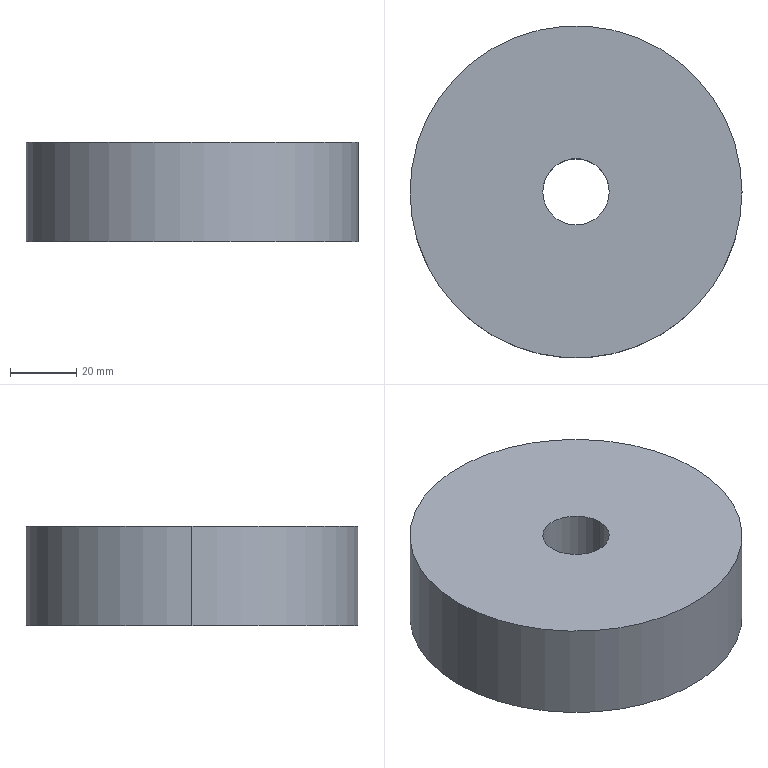Part | STEP file | 1 solid | 6 faces | box 100 x 100 x 30 mm | volume 226195 mm3 | cylinder 4 | plane 2 | commonest cylinder face diameters 20 x2 100 x2
STEP:
#1=CARTESIAN_POINT('',(0.,0.,0.));
#2=DIRECTION('',(0.,0.,1.));
#3=DIRECTION('',(1.,0.,0.));
#4=AXIS2_PLACEMENT_3D('',#1,#2,#3);
#5=CARTESIAN_POINT('',(50.,0.,-15.));
#6=VERTEX_POINT('',#5);
#7=CARTESIAN_POINT('',(-50.,0.,-15.));
#8=VERTEX_POINT('',#7);
#9=CARTESIAN_POINT('',(0.,0.,-15.));
#10=DIRECTION('',(0.,0.,1.));
#11=DIRECTION('',(1.,0.,0.));
#12=AXIS2_PLACEMENT_3D('',#9,#10,#11);
#13=CIRCLE('',#12,50.);
#14=CARTESIAN_POINT('',(0.,0.,0.));
#15=DIRECTION('',(0.,0.,1.));
#16=DIRECTION('',(1.,0.,0.));
#17=AXIS2_PLACEMENT_3D('',#14,#15,#16);
#18=CYLINDRICAL_SURFACE('',#17,50.);
#19=CARTESIAN_POINT('',(0.,-15.));
#20=DIRECTION('',(1.,0.));
#21=VECTOR('',#20,1.);
#22=LINE('',#19,#21);
#23=(GEOMETRIC_REPRESENTATION_CONTEXT(2)PARAMETRIC_REPRESENTATION_CONTEXT()REPRESENTATION_CONTEXT('',''));
#24=DEFINITIONAL_REPRESENTATION('',(#22),#23);
#25=PCURVE('',#18,#24);
#26=CARTESIAN_POINT('',(0.,0.,-15.));
#27=DIRECTION('',(0.,0.,1.));
#28=DIRECTION('',(1.,0.,0.));
#29=AXIS2_PLACEMENT_3D('',#26,#27,#28);
#30=PLANE('',#29);
#31=CARTESIAN_POINT('',(0.,0.));
#32=DIRECTION('',(1.,0.));
#33=AXIS2_PLACEMENT_2D('',#31,#32);
#34=CIRCLE('',#33,50.);
#35=(GEOMETRIC_REPRESENTATION_CONTEXT(2)PARAMETRIC_REPRESENTATION_CONTEXT()REPRESENTATION_CONTEXT('',''));
#36=DEFINITIONAL_REPRESENTATION('',(#34),#35);
#37=PCURVE('',#30,#36);
#38=SURFACE_CURVE('',#13,(#25,#37),.PCURVE_S1.);
#39=EDGE_CURVE('',#6,#8,#38,.T.);
#40=ORIENTED_EDGE('',*,*,#39,.T.);
#41=CARTESIAN_POINT('',(-50.,0.,15.));
#42=VERTEX_POINT('',#41);
#43=CARTESIAN_POINT('',(-50.,0.,0.));
#44=DIRECTION('',(0.,0.,1.));
#45=VECTOR('',#44,1.);
#46=LINE('',#43,#45);
#47=CARTESIAN_POINT('',(3.142,0.));
#48=DIRECTION('',(0.,1.));
#49=VECTOR('',#48,1.);
#50=LINE('',#47,#49);
#51=(GEOMETRIC_REPRESENTATION_CONTEXT(2)PARAMETRIC_REPRESENTATION_CONTEXT()REPRESENTATION_CONTEXT('',''));
#52=DEFINITIONAL_REPRESENTATION('',(#50),#51);
#53=PCURVE('',#18,#52);
#54=CARTESIAN_POINT('',(0.,0.,0.));
#55=DIRECTION('',(0.,0.,1.));
#56=DIRECTION('',(1.,0.,0.));
#57=AXIS2_PLACEMENT_3D('',#54,#55,#56);
#58=CYLINDRICAL_SURFACE('',#57,50.);
#59=CARTESIAN_POINT('',(3.142,0.));
#60=DIRECTION('',(0.,1.));
#61=VECTOR('',#60,1.);
#62=LINE('',#59,#61);
#63=(GEOMETRIC_REPRESENTATION_CONTEXT(2)PARAMETRIC_REPRESENTATION_CONTEXT()REPRESENTATION_CONTEXT('',''));
#64=DEFINITIONAL_REPRESENTATION('',(#62),#63);
#65=PCURVE('',#58,#64);
#66=SURFACE_CURVE('',#46,(#53,#65),.PCURVE_S1.);
#67=EDGE_CURVE('',#8,#42,#66,.T.);
#68=ORIENTED_EDGE('',*,*,#67,.T.);
#69=CARTESIAN_POINT('',(50.,0.,15.));
#70=VERTEX_POINT('',#69);
#71=CARTESIAN_POINT('',(0.,0.,15.));
#72=DIRECTION('',(0.,0.,-1.));
#73=DIRECTION('',(1.,0.,0.));
#74=AXIS2_PLACEMENT_3D('',#71,#72,#73);
#75=CIRCLE('',#74,50.);
#76=CARTESIAN_POINT('',(6.283,15.));
#77=DIRECTION('',(-1.,0.));
#78=VECTOR('',#77,1.);
#79=LINE('',#76,#78);
#80=(GEOMETRIC_REPRESENTATION_CONTEXT(2)PARAMETRIC_REPRESENTATION_CONTEXT()REPRESENTATION_CONTEXT('',''));
#81=DEFINITIONAL_REPRESENTATION('',(#79),#80);
#82=PCURVE('',#18,#81);
#83=CARTESIAN_POINT('',(0.,0.,15.));
#84=DIRECTION('',(0.,0.,1.));
#85=DIRECTION('',(1.,0.,0.));
#86=AXIS2_PLACEMENT_3D('',#83,#84,#85);
#87=PLANE('',#86);
#88=CARTESIAN_POINT('',(50.,0.));
#89=CARTESIAN_POINT('',(50.,-86.603));
#90=CARTESIAN_POINT('',(-25.,-43.301));
#91=CARTESIAN_POINT('',(-100.,0.));
#92=CARTESIAN_POINT('',(-25.,43.301));
#93=CARTESIAN_POINT('',(50.,86.603));
#94=CARTESIAN_POINT('',(50.,0.));
#95=(BOUNDED_CURVE()B_SPLINE_CURVE(2,(#88,#89,#90,#91,#92,#93,#94),.UNSPECIFIED.,.T.,.F.)B_SPLINE_CURVE_WITH_KNOTS((1,2,2,2,2,1),(-2.094,0.,2.094,4.189,6.283,8.378),.UNSPECIFIED.)CURVE()GEOMETRIC_REPRESENTATION_ITEM()RATIONAL_B_SPLINE_CURVE((1.,0.5,1.,0.5,1.,0.5,1.))REPRESENTATION_ITEM(''));
#96=(GEOMETRIC_REPRESENTATION_CONTEXT(2)PARAMETRIC_REPRESENTATION_CONTEXT()REPRESENTATION_CONTEXT('',''));
#97=DEFINITIONAL_REPRESENTATION('',(#95),#96);
#98=PCURVE('',#87,#97);
#99=SURFACE_CURVE('',#75,(#82,#98),.PCURVE_S1.);
#100=EDGE_CURVE('',#42,#70,#99,.T.);
#101=ORIENTED_EDGE('',*,*,#100,.T.);
#102=CARTESIAN_POINT('',(50.,0.,0.));
#103=DIRECTION('',(0.,0.,1.));
#104=VECTOR('',#103,1.);
#105=LINE('',#102,#104);
#106=CARTESIAN_POINT('',(0.,0.));
#107=DIRECTION('',(0.,1.));
#108=VECTOR('',#107,1.);
#109=LINE('',#106,#108);
#110=(GEOMETRIC_REPRESENTATION_CONTEXT(2)PARAMETRIC_REPRESENTATION_CONTEXT()REPRESENTATION_CONTEXT('',''));
#111=DEFINITIONAL_REPRESENTATION('',(#109),#110);
#112=PCURVE('',#18,#111);
#113=CARTESIAN_POINT('',(6.283,0.));
#114=DIRECTION('',(0.,1.));
#115=VECTOR('',#114,1.);
#116=LINE('',#113,#115);
#117=(GEOMETRIC_REPRESENTATION_CONTEXT(2)PARAMETRIC_REPRESENTATION_CONTEXT()REPRESENTATION_CONTEXT('',''));
#118=DEFINITIONAL_REPRESENTATION('',(#116),#117);
#119=PCURVE('',#58,#118);
#120=SURFACE_CURVE('',#105,(#112,#119),.PCURVE_S1.);
#121=EDGE_CURVE('',#6,#70,#120,.T.);
#122=ORIENTED_EDGE('',*,*,#121,.F.);
#123=EDGE_LOOP('',(#40,#68,#101,#122));
#124=FACE_BOUND('',#123,.T.);
#125=ADVANCED_FACE('',(#124),#18,.T.);
#126=CARTESIAN_POINT('',(-10.,0.,15.));
#127=VERTEX_POINT('',#126);
#128=CARTESIAN_POINT('',(-10.,0.,-15.));
#129=VERTEX_POINT('',#128);
#130=CARTESIAN_POINT('',(-10.,0.,15.));
#131=DIRECTION('',(0.,0.,-1.));
#132=VECTOR('',#131,1.);
#133=LINE('',#130,#132);
#134=CARTESIAN_POINT('',(0.,0.,15.));
#135=DIRECTION('',(0.,0.,-1.));
#136=DIRECTION('',(-1.,0.,0.));
#137=AXIS2_PLACEMENT_3D('',#134,#135,#136);
#138=CYLINDRICAL_SURFACE('',#137,10.);
#139=CARTESIAN_POINT('',(6.283,0.));
#140=DIRECTION('',(0.,1.));
#141=VECTOR('',#140,1.);
#142=LINE('',#139,#141);
#143=(GEOMETRIC_REPRESENTATION_CONTEXT(2)PARAMETRIC_REPRESENTATION_CONTEXT()REPRESENTATION_CONTEXT('',''));
#144=DEFINITIONAL_REPRESENTATION('',(#142),#143);
#145=PCURVE('',#138,#144);
#146=CARTESIAN_POINT('',(0.,0.,15.));
#147=DIRECTION('',(0.,0.,-1.));
#148=DIRECTION('',(-1.,0.,0.));
#149=AXIS2_PLACEMENT_3D('',#146,#147,#148);
#150=CYLINDRICAL_SURFACE('',#149,10.);
#151=CARTESIAN_POINT('',(0.,0.));
#152=DIRECTION('',(0.,1.));
#153=VECTOR('',#152,1.);
#154=LINE('',#151,#153);
#155=(GEOMETRIC_REPRESENTATION_CONTEXT(2)PARAMETRIC_REPRESENTATION_CONTEXT()REPRESENTATION_CONTEXT('',''));
#156=DEFINITIONAL_REPRESENTATION('',(#154),#155);
#157=PCURVE('',#150,#156);
#158=SURFACE_CURVE('',#133,(#145,#157),.PCURVE_S1.);
#159=EDGE_CURVE('',#127,#129,#158,.T.);
#160=ORIENTED_EDGE('',*,*,#159,.T.);
#161=CARTESIAN_POINT('',(10.,0.,-15.));
#162=VERTEX_POINT('',#161);
#163=CARTESIAN_POINT('',(0.,0.,-15.));
#164=DIRECTION('',(0.,0.,-1.));
#165=DIRECTION('',(-1.,0.,0.));
#166=AXIS2_PLACEMENT_3D('',#163,#164,#165);
#167=CIRCLE('',#166,10.);
#168=CARTESIAN_POINT('',(0.,30.));
#169=DIRECTION('',(1.,0.));
#170=VECTOR('',#169,1.);
#171=LINE('',#168,#170);
#172=(GEOMETRIC_REPRESENTATION_CONTEXT(2)PARAMETRIC_REPRESENTATION_CONTEXT()REPRESENTATION_CONTEXT('',''));
#173=DEFINITIONAL_REPRESENTATION('',(#171),#172);
#174=PCURVE('',#138,#173);
#175=CARTESIAN_POINT('',(-10.,0.));
#176=CARTESIAN_POINT('',(-10.,17.321));
#177=CARTESIAN_POINT('',(5.,8.66));
#178=CARTESIAN_POINT('',(20.,0.));
#179=CARTESIAN_POINT('',(5.,-8.66));
#180=CARTESIAN_POINT('',(-10.,-17.321));
#181=CARTESIAN_POINT('',(-10.,0.));
#182=(BOUNDED_CURVE()B_SPLINE_CURVE(2,(#175,#176,#177,#178,#179,#180,#181),.UNSPECIFIED.,.T.,.F.)B_SPLINE_CURVE_WITH_KNOTS((1,2,2,2,2,1),(-2.094,0.,2.094,4.189,6.283,8.378),.UNSPECIFIED.)CURVE()GEOMETRIC_REPRESENTATION_ITEM()RATIONAL_B_SPLINE_CURVE((1.,0.5,1.,0.5,1.,0.5,1.))REPRESENTATION_ITEM(''));
#183=(GEOMETRIC_REPRESENTATION_CONTEXT(2)PARAMETRIC_REPRESENTATION_CONTEXT()REPRESENTATION_CONTEXT('',''));
#184=DEFINITIONAL_REPRESENTATION('',(#182),#183);
#185=PCURVE('',#30,#184);
#186=SURFACE_CURVE('',#167,(#174,#185),.PCURVE_S1.);
#187=EDGE_CURVE('',#162,#129,#186,.T.);
#188=ORIENTED_EDGE('',*,*,#187,.F.);
#189=CARTESIAN_POINT('',(10.,0.,15.));
#190=VERTEX_POINT('',#189);
#191=CARTESIAN_POINT('',(10.,0.,15.));
#192=DIRECTION('',(0.,0.,-1.));
#193=VECTOR('',#192,1.);
#194=LINE('',#191,#193);
#195=CARTESIAN_POINT('',(3.142,0.));
#196=DIRECTION('',(0.,1.));
#197=VECTOR('',#196,1.);
#198=LINE('',#195,#197);
#199=(GEOMETRIC_REPRESENTATION_CONTEXT(2)PARAMETRIC_REPRESENTATION_CONTEXT()REPRESENTATION_CONTEXT('',''));
#200=DEFINITIONAL_REPRESENTATION('',(#198),#199);
#201=PCURVE('',#138,#200);
#202=CARTESIAN_POINT('',(3.142,0.));
#203=DIRECTION('',(0.,1.));
#204=VECTOR('',#203,1.);
#205=LINE('',#202,#204);
#206=(GEOMETRIC_REPRESENTATION_CONTEXT(2)PARAMETRIC_REPRESENTATION_CONTEXT()REPRESENTATION_CONTEXT('',''));
#207=DEFINITIONAL_REPRESENTATION('',(#205),#206);
#208=PCURVE('',#150,#207);
#209=SURFACE_CURVE('',#194,(#201,#208),.PCURVE_S1.);
#210=EDGE_CURVE('',#190,#162,#209,.T.);
#211=ORIENTED_EDGE('',*,*,#210,.F.);
#212=CARTESIAN_POINT('',(0.,0.,15.));
#213=DIRECTION('',(0.,0.,-1.));
#214=DIRECTION('',(-1.,0.,0.));
#215=AXIS2_PLACEMENT_3D('',#212,#213,#214);
#216=CIRCLE('',#215,10.);
#217=CARTESIAN_POINT('',(0.,0.));
#218=DIRECTION('',(1.,0.));
#219=VECTOR('',#218,1.);
#220=LINE('',#217,#219);
#221=(GEOMETRIC_REPRESENTATION_CONTEXT(2)PARAMETRIC_REPRESENTATION_CONTEXT()REPRESENTATION_CONTEXT('',''));
#222=DEFINITIONAL_REPRESENTATION('',(#220),#221);
#223=PCURVE('',#138,#222);
#224=CARTESIAN_POINT('',(-10.,0.));
#225=CARTESIAN_POINT('',(-10.,17.321));
#226=CARTESIAN_POINT('',(5.,8.66));
#227=CARTESIAN_POINT('',(20.,0.));
#228=CARTESIAN_POINT('',(5.,-8.66));
#229=CARTESIAN_POINT('',(-10.,-17.321));
#230=CARTESIAN_POINT('',(-10.,0.));
#231=(BOUNDED_CURVE()B_SPLINE_CURVE(2,(#224,#225,#226,#227,#228,#229,#230),.UNSPECIFIED.,.T.,.F.)B_SPLINE_CURVE_WITH_KNOTS((1,2,2,2,2,1),(-2.094,0.,2.094,4.189,6.283,8.378),.UNSPECIFIED.)CURVE()GEOMETRIC_REPRESENTATION_ITEM()RATIONAL_B_SPLINE_CURVE((1.,0.5,1.,0.5,1.,0.5,1.))REPRESENTATION_ITEM(''));
#232=(GEOMETRIC_REPRESENTATION_CONTEXT(2)PARAMETRIC_REPRESENTATION_CONTEXT()REPRESENTATION_CONTEXT('',''));
#233=DEFINITIONAL_REPRESENTATION('',(#231),#232);
#234=PCURVE('',#87,#233);
#235=SURFACE_CURVE('',#216,(#223,#234),.PCURVE_S1.);
#236=EDGE_CURVE('',#190,#127,#235,.T.);
#237=ORIENTED_EDGE('',*,*,#236,.T.);
#238=EDGE_LOOP('',(#160,#188,#211,#237));
#239=FACE_BOUND('',#238,.F.);
#240=ADVANCED_FACE('',(#239),#138,.F.);
#241=ORIENTED_EDGE('',*,*,#67,.F.);
#242=CARTESIAN_POINT('',(0.,0.,-15.));
#243=DIRECTION('',(0.,0.,1.));
#244=DIRECTION('',(1.,0.,0.));
#245=AXIS2_PLACEMENT_3D('',#242,#243,#244);
#246=CIRCLE('',#245,50.);
#247=CARTESIAN_POINT('',(0.,-15.));
#248=DIRECTION('',(1.,0.));
#249=VECTOR('',#248,1.);
#250=LINE('',#247,#249);
#251=(GEOMETRIC_REPRESENTATION_CONTEXT(2)PARAMETRIC_REPRESENTATION_CONTEXT()REPRESENTATION_CONTEXT('',''));
#252=DEFINITIONAL_REPRESENTATION('',(#250),#251);
#253=PCURVE('',#58,#252);
#254=CARTESIAN_POINT('',(0.,0.));
#255=DIRECTION('',(1.,0.));
#256=AXIS2_PLACEMENT_2D('',#254,#255);
#257=CIRCLE('',#256,50.);
#258=(GEOMETRIC_REPRESENTATION_CONTEXT(2)PARAMETRIC_REPRESENTATION_CONTEXT()REPRESENTATION_CONTEXT('',''));
#259=DEFINITIONAL_REPRESENTATION('',(#257),#258);
#260=PCURVE('',#30,#259);
#261=SURFACE_CURVE('',#246,(#253,#260),.PCURVE_S1.);
#262=EDGE_CURVE('',#8,#6,#261,.T.);
#263=ORIENTED_EDGE('',*,*,#262,.T.);
#264=ORIENTED_EDGE('',*,*,#121,.T.);
#265=CARTESIAN_POINT('',(0.,0.,15.));
#266=DIRECTION('',(0.,0.,-1.));
#267=DIRECTION('',(1.,0.,0.));
#268=AXIS2_PLACEMENT_3D('',#265,#266,#267);
#269=CIRCLE('',#268,50.);
#270=CARTESIAN_POINT('',(6.283,15.));
#271=DIRECTION('',(-1.,0.));
#272=VECTOR('',#271,1.);
#273=LINE('',#270,#272);
#274=(GEOMETRIC_REPRESENTATION_CONTEXT(2)PARAMETRIC_REPRESENTATION_CONTEXT()REPRESENTATION_CONTEXT('',''));
#275=DEFINITIONAL_REPRESENTATION('',(#273),#274);
#276=PCURVE('',#58,#275);
#277=CARTESIAN_POINT('',(50.,0.));
#278=CARTESIAN_POINT('',(50.,-86.603));
#279=CARTESIAN_POINT('',(-25.,-43.301));
#280=CARTESIAN_POINT('',(-100.,0.));
#281=CARTESIAN_POINT('',(-25.,43.301));
#282=CARTESIAN_POINT('',(50.,86.603));
#283=CARTESIAN_POINT('',(50.,0.));
#284=(BOUNDED_CURVE()B_SPLINE_CURVE(2,(#277,#278,#279,#280,#281,#282,#283),.UNSPECIFIED.,.T.,.F.)B_SPLINE_CURVE_WITH_KNOTS((1,2,2,2,2,1),(-2.094,0.,2.094,4.189,6.283,8.378),.UNSPECIFIED.)CURVE()GEOMETRIC_REPRESENTATION_ITEM()RATIONAL_B_SPLINE_CURVE((1.,0.5,1.,0.5,1.,0.5,1.))REPRESENTATION_ITEM(''));
#285=(GEOMETRIC_REPRESENTATION_CONTEXT(2)PARAMETRIC_REPRESENTATION_CONTEXT()REPRESENTATION_CONTEXT('',''));
#286=DEFINITIONAL_REPRESENTATION('',(#284),#285);
#287=PCURVE('',#87,#286);
#288=SURFACE_CURVE('',#269,(#276,#287),.PCURVE_S1.);
#289=EDGE_CURVE('',#70,#42,#288,.T.);
#290=ORIENTED_EDGE('',*,*,#289,.T.);
#291=EDGE_LOOP('',(#241,#263,#264,#290));
#292=FACE_BOUND('',#291,.T.);
#293=ADVANCED_FACE('',(#292),#58,.T.);
#294=ORIENTED_EDGE('',*,*,#289,.F.);
#295=ORIENTED_EDGE('',*,*,#100,.F.);
#296=EDGE_LOOP('',(#294,#295));
#297=FACE_BOUND('',#296,.T.);
#298=CARTESIAN_POINT('',(0.,0.,15.));
#299=DIRECTION('',(0.,0.,-1.));
#300=DIRECTION('',(-1.,0.,0.));
#301=AXIS2_PLACEMENT_3D('',#298,#299,#300);
#302=CIRCLE('',#301,10.);
#303=CARTESIAN_POINT('',(-10.,0.));
#304=CARTESIAN_POINT('',(-10.,17.321));
#305=CARTESIAN_POINT('',(5.,8.66));
#306=CARTESIAN_POINT('',(20.,0.));
#307=CARTESIAN_POINT('',(5.,-8.66));
#308=CARTESIAN_POINT('',(-10.,-17.321));
#309=CARTESIAN_POINT('',(-10.,0.));
#310=(BOUNDED_CURVE()B_SPLINE_CURVE(2,(#303,#304,#305,#306,#307,#308,#309),.UNSPECIFIED.,.T.,.F.)B_SPLINE_CURVE_WITH_KNOTS((1,2,2,2,2,1),(-2.094,0.,2.094,4.189,6.283,8.378),.UNSPECIFIED.)CURVE()GEOMETRIC_REPRESENTATION_ITEM()RATIONAL_B_SPLINE_CURVE((1.,0.5,1.,0.5,1.,0.5,1.))REPRESENTATION_ITEM(''));
#311=(GEOMETRIC_REPRESENTATION_CONTEXT(2)PARAMETRIC_REPRESENTATION_CONTEXT()REPRESENTATION_CONTEXT('',''));
#312=DEFINITIONAL_REPRESENTATION('',(#310),#311);
#313=PCURVE('',#87,#312);
#314=CARTESIAN_POINT('',(0.,0.));
#315=DIRECTION('',(1.,0.));
#316=VECTOR('',#315,1.);
#317=LINE('',#314,#316);
#318=(GEOMETRIC_REPRESENTATION_CONTEXT(2)PARAMETRIC_REPRESENTATION_CONTEXT()REPRESENTATION_CONTEXT('',''));
#319=DEFINITIONAL_REPRESENTATION('',(#317),#318);
#320=PCURVE('',#150,#319);
#321=SURFACE_CURVE('',#302,(#313,#320),.PCURVE_S1.);
#322=EDGE_CURVE('',#127,#190,#321,.T.);
#323=ORIENTED_EDGE('',*,*,#322,.T.);
#324=ORIENTED_EDGE('',*,*,#236,.T.);
#325=EDGE_LOOP('',(#323,#324));
#326=FACE_BOUND('',#325,.T.);
#327=ADVANCED_FACE('',(#297,#326),#87,.T.);
#328=ORIENTED_EDGE('',*,*,#39,.F.);
#329=ORIENTED_EDGE('',*,*,#262,.F.);
#330=EDGE_LOOP('',(#328,#329));
#331=FACE_BOUND('',#330,.T.);
#332=CARTESIAN_POINT('',(0.,0.,-15.));
#333=DIRECTION('',(0.,0.,-1.));
#334=DIRECTION('',(-1.,0.,0.));
#335=AXIS2_PLACEMENT_3D('',#332,#333,#334);
#336=CIRCLE('',#335,10.);
#337=CARTESIAN_POINT('',(-10.,0.));
#338=CARTESIAN_POINT('',(-10.,17.321));
#339=CARTESIAN_POINT('',(5.,8.66));
#340=CARTESIAN_POINT('',(20.,0.));
#341=CARTESIAN_POINT('',(5.,-8.66));
#342=CARTESIAN_POINT('',(-10.,-17.321));
#343=CARTESIAN_POINT('',(-10.,0.));
#344=(BOUNDED_CURVE()B_SPLINE_CURVE(2,(#337,#338,#339,#340,#341,#342,#343),.UNSPECIFIED.,.T.,.F.)B_SPLINE_CURVE_WITH_KNOTS((1,2,2,2,2,1),(-2.094,0.,2.094,4.189,6.283,8.378),.UNSPECIFIED.)CURVE()GEOMETRIC_REPRESENTATION_ITEM()RATIONAL_B_SPLINE_CURVE((1.,0.5,1.,0.5,1.,0.5,1.))REPRESENTATION_ITEM(''));
#345=(GEOMETRIC_REPRESENTATION_CONTEXT(2)PARAMETRIC_REPRESENTATION_CONTEXT()REPRESENTATION_CONTEXT('',''));
#346=DEFINITIONAL_REPRESENTATION('',(#344),#345);
#347=PCURVE('',#30,#346);
#348=CARTESIAN_POINT('',(0.,30.));
#349=DIRECTION('',(1.,0.));
#350=VECTOR('',#349,1.);
#351=LINE('',#348,#350);
#352=(GEOMETRIC_REPRESENTATION_CONTEXT(2)PARAMETRIC_REPRESENTATION_CONTEXT()REPRESENTATION_CONTEXT('',''));
#353=DEFINITIONAL_REPRESENTATION('',(#351),#352);
#354=PCURVE('',#150,#353);
#355=SURFACE_CURVE('',#336,(#347,#354),.PCURVE_S1.);
#356=EDGE_CURVE('',#129,#162,#355,.T.);
#357=ORIENTED_EDGE('',*,*,#356,.F.);
#358=ORIENTED_EDGE('',*,*,#187,.F.);
#359=EDGE_LOOP('',(#357,#358));
#360=FACE_BOUND('',#359,.T.);
#361=ADVANCED_FACE('',(#331,#360),#30,.F.);
#362=ORIENTED_EDGE('',*,*,#356,.F.);
#363=ORIENTED_EDGE('',*,*,#159,.F.);
#364=ORIENTED_EDGE('',*,*,#322,.T.);
#365=ORIENTED_EDGE('',*,*,#210,.T.);
#366=EDGE_LOOP('',(#362,#363,#364,#365));
#367=FACE_BOUND('',#366,.F.);
#368=ADVANCED_FACE('',(#367),#150,.F.);
#369=CLOSED_SHELL('',(#125,#240,#293,#327,#361,#368));
#370=MANIFOLD_SOLID_BREP('',#369);
#371=(LENGTH_UNIT()NAMED_UNIT(*)SI_UNIT(.MILLI.,.METRE.));
#372=UNCERTAINTY_MEASURE_WITH_UNIT(LENGTH_MEASURE(0.0000001),#371,'','');
#373=(NAMED_UNIT(*)PLANE_ANGLE_UNIT()SI_UNIT($,.RADIAN.));
#374=(NAMED_UNIT(*)SI_UNIT($,.STERADIAN.)SOLID_ANGLE_UNIT());
#375=(GEOMETRIC_REPRESENTATION_CONTEXT(3)GLOBAL_UNCERTAINTY_ASSIGNED_CONTEXT((#372))GLOBAL_UNIT_ASSIGNED_CONTEXT((#371,#373,#374))REPRESENTATION_CONTEXT('',''));
#376=ADVANCED_BREP_SHAPE_REPRESENTATION('',(#4,#370),#375);